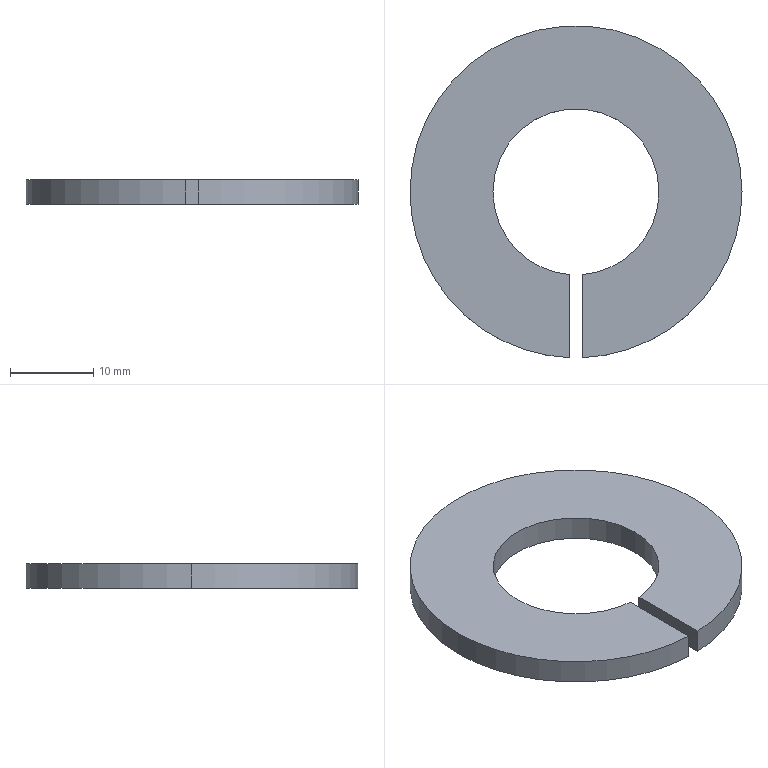Part | STEP file | qnSceond3_2 | 1 solid | 10 faces | box 40 x 39.986 x 3 mm | volume 2782 mm3 | cylinder 6 | plane 4 | commonest cylinder face diameters 20 x3 40 x3
STEP:
#1=CARTESIAN_POINT('',(0.,0.,0.));
#2=DIRECTION('',(0.,0.,1.));
#3=DIRECTION('',(1.,0.,0.));
#4=AXIS2_PLACEMENT_3D('',#1,#2,#3);
#5=CARTESIAN_POINT('',(20.,0.,8.));
#6=VERTEX_POINT('',#5);
#7=CARTESIAN_POINT('',(-20.,0.,8.));
#8=VERTEX_POINT('',#7);
#9=CARTESIAN_POINT('',(0.,0.,8.));
#10=DIRECTION('',(0.,0.,1.));
#11=DIRECTION('',(-1.,0.,0.));
#12=AXIS2_PLACEMENT_3D('',#9,#10,#11);
#13=CIRCLE('',#12,20.);
#14=CARTESIAN_POINT('',(0.,0.,6.5));
#15=DIRECTION('',(0.,0.,-1.));
#16=DIRECTION('',(-1.,0.,0.));
#17=AXIS2_PLACEMENT_3D('',#14,#15,#16);
#18=CYLINDRICAL_SURFACE('',#17,20.);
#19=CARTESIAN_POINT('',(6.283,-1.5));
#20=DIRECTION('',(-1.,0.));
#21=VECTOR('',#20,1.);
#22=LINE('',#19,#21);
#23=(GEOMETRIC_REPRESENTATION_CONTEXT(2)PARAMETRIC_REPRESENTATION_CONTEXT()REPRESENTATION_CONTEXT('',''));
#24=DEFINITIONAL_REPRESENTATION('',(#22),#23);
#25=PCURVE('',#18,#24);
#26=CARTESIAN_POINT('',(0.,15.,8.));
#27=DIRECTION('',(0.,0.,1.));
#28=DIRECTION('',(1.,0.,0.));
#29=AXIS2_PLACEMENT_3D('',#26,#27,#28);
#30=PLANE('',#29);
#31=CARTESIAN_POINT('',(0.,-15.));
#32=DIRECTION('',(-1.,0.));
#33=AXIS2_PLACEMENT_2D('',#31,#32);
#34=CIRCLE('',#33,20.);
#35=(GEOMETRIC_REPRESENTATION_CONTEXT(2)PARAMETRIC_REPRESENTATION_CONTEXT()REPRESENTATION_CONTEXT('',''));
#36=DEFINITIONAL_REPRESENTATION('',(#34),#35);
#37=PCURVE('',#30,#36);
#38=SURFACE_CURVE('',#13,(#25,#37),.PCURVE_S1.);
#39=EDGE_CURVE('',#6,#8,#38,.T.);
#40=ORIENTED_EDGE('',*,*,#39,.F.);
#41=CARTESIAN_POINT('',(20.,0.,5.));
#42=VERTEX_POINT('',#41);
#43=CARTESIAN_POINT('',(20.,0.,6.5));
#44=DIRECTION('',(0.,0.,-1.));
#45=VECTOR('',#44,1.);
#46=LINE('',#43,#45);
#47=CARTESIAN_POINT('',(3.142,0.));
#48=DIRECTION('',(0.,1.));
#49=VECTOR('',#48,1.);
#50=LINE('',#47,#49);
#51=(GEOMETRIC_REPRESENTATION_CONTEXT(2)PARAMETRIC_REPRESENTATION_CONTEXT()REPRESENTATION_CONTEXT('',''));
#52=DEFINITIONAL_REPRESENTATION('',(#50),#51);
#53=PCURVE('',#18,#52);
#54=CARTESIAN_POINT('',(0.,0.,6.5));
#55=DIRECTION('',(0.,0.,-1.));
#56=DIRECTION('',(-1.,0.,0.));
#57=AXIS2_PLACEMENT_3D('',#54,#55,#56);
#58=CYLINDRICAL_SURFACE('',#57,20.);
#59=CARTESIAN_POINT('',(3.142,0.));
#60=DIRECTION('',(0.,1.));
#61=VECTOR('',#60,1.);
#62=LINE('',#59,#61);
#63=(GEOMETRIC_REPRESENTATION_CONTEXT(2)PARAMETRIC_REPRESENTATION_CONTEXT()REPRESENTATION_CONTEXT('',''));
#64=DEFINITIONAL_REPRESENTATION('',(#62),#63);
#65=PCURVE('',#58,#64);
#66=SURFACE_CURVE('',#46,(#53,#65),.PCURVE_S1.);
#67=EDGE_CURVE('',#6,#42,#66,.T.);
#68=ORIENTED_EDGE('',*,*,#67,.T.);
#69=CARTESIAN_POINT('',(-20.,0.,5.));
#70=VERTEX_POINT('',#69);
#71=CARTESIAN_POINT('',(0.,0.,5.));
#72=DIRECTION('',(0.,0.,1.));
#73=DIRECTION('',(-1.,0.,0.));
#74=AXIS2_PLACEMENT_3D('',#71,#72,#73);
#75=CIRCLE('',#74,20.);
#76=CARTESIAN_POINT('',(6.283,1.5));
#77=DIRECTION('',(-1.,0.));
#78=VECTOR('',#77,1.);
#79=LINE('',#76,#78);
#80=(GEOMETRIC_REPRESENTATION_CONTEXT(2)PARAMETRIC_REPRESENTATION_CONTEXT()REPRESENTATION_CONTEXT('',''));
#81=DEFINITIONAL_REPRESENTATION('',(#79),#80);
#82=PCURVE('',#18,#81);
#83=CARTESIAN_POINT('',(0.,15.,5.));
#84=DIRECTION('',(0.,0.,-1.));
#85=DIRECTION('',(-1.,0.,0.));
#86=AXIS2_PLACEMENT_3D('',#83,#84,#85);
#87=PLANE('',#86);
#88=CARTESIAN_POINT('',(20.,-15.));
#89=CARTESIAN_POINT('',(20.,-49.641));
#90=CARTESIAN_POINT('',(-10.,-32.321));
#91=CARTESIAN_POINT('',(-40.,-15.));
#92=CARTESIAN_POINT('',(-10.,2.321));
#93=CARTESIAN_POINT('',(20.,19.641));
#94=CARTESIAN_POINT('',(20.,-15.));
#95=(BOUNDED_CURVE()B_SPLINE_CURVE(2,(#88,#89,#90,#91,#92,#93,#94),.UNSPECIFIED.,.T.,.F.)B_SPLINE_CURVE_WITH_KNOTS((1,2,2,2,2,1),(-2.094,0.,2.094,4.189,6.283,8.378),.UNSPECIFIED.)CURVE()GEOMETRIC_REPRESENTATION_ITEM()RATIONAL_B_SPLINE_CURVE((1.,0.5,1.,0.5,1.,0.5,1.))REPRESENTATION_ITEM(''));
#96=(GEOMETRIC_REPRESENTATION_CONTEXT(2)PARAMETRIC_REPRESENTATION_CONTEXT()REPRESENTATION_CONTEXT('',''));
#97=DEFINITIONAL_REPRESENTATION('',(#95),#96);
#98=PCURVE('',#87,#97);
#99=SURFACE_CURVE('',#75,(#82,#98),.PCURVE_S1.);
#100=EDGE_CURVE('',#42,#70,#99,.T.);
#101=ORIENTED_EDGE('',*,*,#100,.T.);
#102=CARTESIAN_POINT('',(-20.,0.,6.5));
#103=DIRECTION('',(0.,0.,-1.));
#104=VECTOR('',#103,1.);
#105=LINE('',#102,#104);
#106=CARTESIAN_POINT('',(0.,0.));
#107=DIRECTION('',(0.,1.));
#108=VECTOR('',#107,1.);
#109=LINE('',#106,#108);
#110=(GEOMETRIC_REPRESENTATION_CONTEXT(2)PARAMETRIC_REPRESENTATION_CONTEXT()REPRESENTATION_CONTEXT('',''));
#111=DEFINITIONAL_REPRESENTATION('',(#109),#110);
#112=PCURVE('',#18,#111);
#113=CARTESIAN_POINT('',(0.,0.,6.5));
#114=DIRECTION('',(0.,0.,-1.));
#115=DIRECTION('',(-1.,0.,0.));
#116=AXIS2_PLACEMENT_3D('',#113,#114,#115);
#117=CYLINDRICAL_SURFACE('',#116,20.);
#118=CARTESIAN_POINT('',(6.283,0.));
#119=DIRECTION('',(0.,1.));
#120=VECTOR('',#119,1.);
#121=LINE('',#118,#120);
#122=(GEOMETRIC_REPRESENTATION_CONTEXT(2)PARAMETRIC_REPRESENTATION_CONTEXT()REPRESENTATION_CONTEXT('',''));
#123=DEFINITIONAL_REPRESENTATION('',(#121),#122);
#124=PCURVE('',#117,#123);
#125=SURFACE_CURVE('',#105,(#112,#124),.PCURVE_S1.);
#126=EDGE_CURVE('',#8,#70,#125,.T.);
#127=ORIENTED_EDGE('',*,*,#126,.F.);
#128=EDGE_LOOP('',(#40,#68,#101,#127));
#129=FACE_BOUND('',#128,.T.);
#130=ADVANCED_FACE('',(#129),#18,.T.);
#131=CARTESIAN_POINT('',(-0.75,-19.986,8.));
#132=VERTEX_POINT('',#131);
#133=CARTESIAN_POINT('',(0.,0.,8.));
#134=DIRECTION('',(0.,0.,1.));
#135=DIRECTION('',(-1.,0.,0.));
#136=AXIS2_PLACEMENT_3D('',#133,#134,#135);
#137=CIRCLE('',#136,20.);
#138=CARTESIAN_POINT('',(6.283,-1.5));
#139=DIRECTION('',(-1.,0.));
#140=VECTOR('',#139,1.);
#141=LINE('',#138,#140);
#142=(GEOMETRIC_REPRESENTATION_CONTEXT(2)PARAMETRIC_REPRESENTATION_CONTEXT()REPRESENTATION_CONTEXT('',''));
#143=DEFINITIONAL_REPRESENTATION('',(#141),#142);
#144=PCURVE('',#117,#143);
#145=CARTESIAN_POINT('',(0.,-15.));
#146=DIRECTION('',(-1.,0.));
#147=AXIS2_PLACEMENT_2D('',#145,#146);
#148=CIRCLE('',#147,20.);
#149=(GEOMETRIC_REPRESENTATION_CONTEXT(2)PARAMETRIC_REPRESENTATION_CONTEXT()REPRESENTATION_CONTEXT('',''));
#150=DEFINITIONAL_REPRESENTATION('',(#148),#149);
#151=PCURVE('',#30,#150);
#152=SURFACE_CURVE('',#137,(#144,#151),.PCURVE_S1.);
#153=EDGE_CURVE('',#8,#132,#152,.T.);
#154=ORIENTED_EDGE('',*,*,#153,.F.);
#155=ORIENTED_EDGE('',*,*,#126,.T.);
#156=CARTESIAN_POINT('',(-0.75,-19.986,5.));
#157=VERTEX_POINT('',#156);
#158=CARTESIAN_POINT('',(0.,0.,5.));
#159=DIRECTION('',(0.,0.,1.));
#160=DIRECTION('',(-1.,0.,0.));
#161=AXIS2_PLACEMENT_3D('',#158,#159,#160);
#162=CIRCLE('',#161,20.);
#163=CARTESIAN_POINT('',(6.283,1.5));
#164=DIRECTION('',(-1.,0.));
#165=VECTOR('',#164,1.);
#166=LINE('',#163,#165);
#167=(GEOMETRIC_REPRESENTATION_CONTEXT(2)PARAMETRIC_REPRESENTATION_CONTEXT()REPRESENTATION_CONTEXT('',''));
#168=DEFINITIONAL_REPRESENTATION('',(#166),#167);
#169=PCURVE('',#117,#168);
#170=CARTESIAN_POINT('',(20.,-15.));
#171=CARTESIAN_POINT('',(20.,-49.641));
#172=CARTESIAN_POINT('',(-10.,-32.321));
#173=CARTESIAN_POINT('',(-40.,-15.));
#174=CARTESIAN_POINT('',(-10.,2.321));
#175=CARTESIAN_POINT('',(20.,19.641));
#176=CARTESIAN_POINT('',(20.,-15.));
#177=(BOUNDED_CURVE()B_SPLINE_CURVE(2,(#170,#171,#172,#173,#174,#175,#176),.UNSPECIFIED.,.T.,.F.)B_SPLINE_CURVE_WITH_KNOTS((1,2,2,2,2,1),(-2.094,0.,2.094,4.189,6.283,8.378),.UNSPECIFIED.)CURVE()GEOMETRIC_REPRESENTATION_ITEM()RATIONAL_B_SPLINE_CURVE((1.,0.5,1.,0.5,1.,0.5,1.))REPRESENTATION_ITEM(''));
#178=(GEOMETRIC_REPRESENTATION_CONTEXT(2)PARAMETRIC_REPRESENTATION_CONTEXT()REPRESENTATION_CONTEXT('',''));
#179=DEFINITIONAL_REPRESENTATION('',(#177),#178);
#180=PCURVE('',#87,#179);
#181=SURFACE_CURVE('',#162,(#169,#180),.PCURVE_S1.);
#182=EDGE_CURVE('',#70,#157,#181,.T.);
#183=ORIENTED_EDGE('',*,*,#182,.T.);
#184=CARTESIAN_POINT('',(-0.75,-19.986,6.5));
#185=DIRECTION('',(0.,0.,1.));
#186=VECTOR('',#185,1.);
#187=LINE('',#184,#186);
#188=CARTESIAN_POINT('',(4.75,0.));
#189=DIRECTION('',(0.,-1.));
#190=VECTOR('',#189,1.);
#191=LINE('',#188,#190);
#192=(GEOMETRIC_REPRESENTATION_CONTEXT(2)PARAMETRIC_REPRESENTATION_CONTEXT()REPRESENTATION_CONTEXT('',''));
#193=DEFINITIONAL_REPRESENTATION('',(#191),#192);
#194=PCURVE('',#117,#193);
#195=CARTESIAN_POINT('',(-0.75,-40.,5.));
#196=DIRECTION('',(-1.,0.,0.));
#197=DIRECTION('',(0.,0.,1.));
#198=AXIS2_PLACEMENT_3D('',#195,#196,#197);
#199=PLANE('',#198);
#200=CARTESIAN_POINT('',(1.5,20.014));
#201=DIRECTION('',(1.,0.));
#202=VECTOR('',#201,1.);
#203=LINE('',#200,#202);
#204=(GEOMETRIC_REPRESENTATION_CONTEXT(2)PARAMETRIC_REPRESENTATION_CONTEXT()REPRESENTATION_CONTEXT('',''));
#205=DEFINITIONAL_REPRESENTATION('',(#203),#204);
#206=PCURVE('',#199,#205);
#207=SURFACE_CURVE('',#187,(#194,#206),.PCURVE_S1.);
#208=EDGE_CURVE('',#157,#132,#207,.T.);
#209=ORIENTED_EDGE('',*,*,#208,.T.);
#210=EDGE_LOOP('',(#154,#155,#183,#209));
#211=FACE_BOUND('',#210,.T.);
#212=ADVANCED_FACE('',(#211),#117,.T.);
#213=CARTESIAN_POINT('',(0.75,-9.972,5.));
#214=VERTEX_POINT('',#213);
#215=CARTESIAN_POINT('',(0.75,-9.972,8.));
#216=VERTEX_POINT('',#215);
#217=CARTESIAN_POINT('',(0.75,-9.972,5.));
#218=DIRECTION('',(0.,0.,1.));
#219=VECTOR('',#218,1.);
#220=LINE('',#217,#219);
#221=CARTESIAN_POINT('',(0.,0.,6.5));
#222=DIRECTION('',(0.,0.,-1.));
#223=DIRECTION('',(-1.,0.,0.));
#224=AXIS2_PLACEMENT_3D('',#221,#222,#223);
#225=CYLINDRICAL_SURFACE('',#224,10.);
#226=CARTESIAN_POINT('',(4.637,1.5));
#227=DIRECTION('',(0.,-1.));
#228=VECTOR('',#227,1.);
#229=LINE('',#226,#228);
#230=(GEOMETRIC_REPRESENTATION_CONTEXT(2)PARAMETRIC_REPRESENTATION_CONTEXT()REPRESENTATION_CONTEXT('',''));
#231=DEFINITIONAL_REPRESENTATION('',(#229),#230);
#232=PCURVE('',#225,#231);
#233=CARTESIAN_POINT('',(0.75,0.,5.));
#234=DIRECTION('',(1.,0.,0.));
#235=DIRECTION('',(0.,0.,-1.));
#236=AXIS2_PLACEMENT_3D('',#233,#234,#235);
#237=PLANE('',#236);
#238=CARTESIAN_POINT('',(0.,-9.972));
#239=DIRECTION('',(-1.,0.));
#240=VECTOR('',#239,1.);
#241=LINE('',#238,#240);
#242=(GEOMETRIC_REPRESENTATION_CONTEXT(2)PARAMETRIC_REPRESENTATION_CONTEXT()REPRESENTATION_CONTEXT('',''));
#243=DEFINITIONAL_REPRESENTATION('',(#241),#242);
#244=PCURVE('',#237,#243);
#245=SURFACE_CURVE('',#220,(#232,#244),.PCURVE_S1.);
#246=EDGE_CURVE('',#214,#216,#245,.T.);
#247=ORIENTED_EDGE('',*,*,#246,.F.);
#248=CARTESIAN_POINT('',(10.,0.,5.));
#249=VERTEX_POINT('',#248);
#250=CARTESIAN_POINT('',(0.,0.,5.));
#251=DIRECTION('',(0.,0.,1.));
#252=DIRECTION('',(-1.,0.,0.));
#253=AXIS2_PLACEMENT_3D('',#250,#251,#252);
#254=CIRCLE('',#253,10.);
#255=CARTESIAN_POINT('',(6.283,1.5));
#256=DIRECTION('',(-1.,0.));
#257=VECTOR('',#256,1.);
#258=LINE('',#255,#257);
#259=(GEOMETRIC_REPRESENTATION_CONTEXT(2)PARAMETRIC_REPRESENTATION_CONTEXT()REPRESENTATION_CONTEXT('',''));
#260=DEFINITIONAL_REPRESENTATION('',(#258),#259);
#261=PCURVE('',#225,#260);
#262=CARTESIAN_POINT('',(10.,-15.));
#263=CARTESIAN_POINT('',(10.,-32.321));
#264=CARTESIAN_POINT('',(-5.,-23.66));
#265=CARTESIAN_POINT('',(-20.,-15.));
#266=CARTESIAN_POINT('',(-5.,-6.34));
#267=CARTESIAN_POINT('',(10.,2.321));
#268=CARTESIAN_POINT('',(10.,-15.));
#269=(BOUNDED_CURVE()B_SPLINE_CURVE(2,(#262,#263,#264,#265,#266,#267,#268),.UNSPECIFIED.,.T.,.F.)B_SPLINE_CURVE_WITH_KNOTS((1,2,2,2,2,1),(-2.094,0.,2.094,4.189,6.283,8.378),.UNSPECIFIED.)CURVE()GEOMETRIC_REPRESENTATION_ITEM()RATIONAL_B_SPLINE_CURVE((1.,0.5,1.,0.5,1.,0.5,1.))REPRESENTATION_ITEM(''));
#270=(GEOMETRIC_REPRESENTATION_CONTEXT(2)PARAMETRIC_REPRESENTATION_CONTEXT()REPRESENTATION_CONTEXT('',''));
#271=DEFINITIONAL_REPRESENTATION('',(#269),#270);
#272=PCURVE('',#87,#271);
#273=SURFACE_CURVE('',#254,(#261,#272),.PCURVE_S1.);
#274=EDGE_CURVE('',#214,#249,#273,.T.);
#275=ORIENTED_EDGE('',*,*,#274,.T.);
#276=CARTESIAN_POINT('',(10.,0.,8.));
#277=VERTEX_POINT('',#276);
#278=CARTESIAN_POINT('',(10.,0.,6.5));
#279=DIRECTION('',(0.,0.,-1.));
#280=VECTOR('',#279,1.);
#281=LINE('',#278,#280);
#282=CARTESIAN_POINT('',(3.142,0.));
#283=DIRECTION('',(0.,1.));
#284=VECTOR('',#283,1.);
#285=LINE('',#282,#284);
#286=(GEOMETRIC_REPRESENTATION_CONTEXT(2)PARAMETRIC_REPRESENTATION_CONTEXT()REPRESENTATION_CONTEXT('',''));
#287=DEFINITIONAL_REPRESENTATION('',(#285),#286);
#288=PCURVE('',#225,#287);
#289=CARTESIAN_POINT('',(0.,0.,6.5));
#290=DIRECTION('',(0.,0.,-1.));
#291=DIRECTION('',(-1.,0.,0.));
#292=AXIS2_PLACEMENT_3D('',#289,#290,#291);
#293=CYLINDRICAL_SURFACE('',#292,10.);
#294=CARTESIAN_POINT('',(3.142,0.));
#295=DIRECTION('',(0.,1.));
#296=VECTOR('',#295,1.);
#297=LINE('',#294,#296);
#298=(GEOMETRIC_REPRESENTATION_CONTEXT(2)PARAMETRIC_REPRESENTATION_CONTEXT()REPRESENTATION_CONTEXT('',''));
#299=DEFINITIONAL_REPRESENTATION('',(#297),#298);
#300=PCURVE('',#293,#299);
#301=SURFACE_CURVE('',#281,(#288,#300),.PCURVE_S1.);
#302=EDGE_CURVE('',#277,#249,#301,.T.);
#303=ORIENTED_EDGE('',*,*,#302,.F.);
#304=CARTESIAN_POINT('',(0.,0.,8.));
#305=DIRECTION('',(0.,0.,-1.));
#306=DIRECTION('',(-1.,0.,0.));
#307=AXIS2_PLACEMENT_3D('',#304,#305,#306);
#308=CIRCLE('',#307,10.);
#309=CARTESIAN_POINT('',(0.,-1.5));
#310=DIRECTION('',(1.,0.));
#311=VECTOR('',#310,1.);
#312=LINE('',#309,#311);
#313=(GEOMETRIC_REPRESENTATION_CONTEXT(2)PARAMETRIC_REPRESENTATION_CONTEXT()REPRESENTATION_CONTEXT('',''));
#314=DEFINITIONAL_REPRESENTATION('',(#312),#313);
#315=PCURVE('',#225,#314);
#316=CARTESIAN_POINT('',(-10.,-15.));
#317=CARTESIAN_POINT('',(-10.,2.321));
#318=CARTESIAN_POINT('',(5.,-6.34));
#319=CARTESIAN_POINT('',(20.,-15.));
#320=CARTESIAN_POINT('',(5.,-23.66));
#321=CARTESIAN_POINT('',(-10.,-32.321));
#322=CARTESIAN_POINT('',(-10.,-15.));
#323=(BOUNDED_CURVE()B_SPLINE_CURVE(2,(#316,#317,#318,#319,#320,#321,#322),.UNSPECIFIED.,.T.,.F.)B_SPLINE_CURVE_WITH_KNOTS((1,2,2,2,2,1),(-2.094,0.,2.094,4.189,6.283,8.378),.UNSPECIFIED.)CURVE()GEOMETRIC_REPRESENTATION_ITEM()RATIONAL_B_SPLINE_CURVE((1.,0.5,1.,0.5,1.,0.5,1.))REPRESENTATION_ITEM(''));
#324=(GEOMETRIC_REPRESENTATION_CONTEXT(2)PARAMETRIC_REPRESENTATION_CONTEXT()REPRESENTATION_CONTEXT('',''));
#325=DEFINITIONAL_REPRESENTATION('',(#323),#324);
#326=PCURVE('',#30,#325);
#327=SURFACE_CURVE('',#308,(#315,#326),.PCURVE_S1.);
#328=EDGE_CURVE('',#277,#216,#327,.T.);
#329=ORIENTED_EDGE('',*,*,#328,.T.);
#330=EDGE_LOOP('',(#247,#275,#303,#329));
#331=FACE_BOUND('',#330,.F.);
#332=ADVANCED_FACE('',(#331),#225,.F.);
#333=CARTESIAN_POINT('',(-10.,0.,5.));
#334=VERTEX_POINT('',#333);
#335=CARTESIAN_POINT('',(0.,0.,5.));
#336=DIRECTION('',(0.,0.,1.));
#337=DIRECTION('',(-1.,0.,0.));
#338=AXIS2_PLACEMENT_3D('',#335,#336,#337);
#339=CIRCLE('',#338,10.);
#340=CARTESIAN_POINT('',(6.283,1.5));
#341=DIRECTION('',(-1.,0.));
#342=VECTOR('',#341,1.);
#343=LINE('',#340,#342);
#344=(GEOMETRIC_REPRESENTATION_CONTEXT(2)PARAMETRIC_REPRESENTATION_CONTEXT()REPRESENTATION_CONTEXT('',''));
#345=DEFINITIONAL_REPRESENTATION('',(#343),#344);
#346=PCURVE('',#293,#345);
#347=CARTESIAN_POINT('',(10.,-15.));
#348=CARTESIAN_POINT('',(10.,-32.321));
#349=CARTESIAN_POINT('',(-5.,-23.66));
#350=CARTESIAN_POINT('',(-20.,-15.));
#351=CARTESIAN_POINT('',(-5.,-6.34));
#352=CARTESIAN_POINT('',(10.,2.321));
#353=CARTESIAN_POINT('',(10.,-15.));
#354=(BOUNDED_CURVE()B_SPLINE_CURVE(2,(#347,#348,#349,#350,#351,#352,#353),.UNSPECIFIED.,.T.,.F.)B_SPLINE_CURVE_WITH_KNOTS((1,2,2,2,2,1),(-2.094,0.,2.094,4.189,6.283,8.378),.UNSPECIFIED.)CURVE()GEOMETRIC_REPRESENTATION_ITEM()RATIONAL_B_SPLINE_CURVE((1.,0.5,1.,0.5,1.,0.5,1.))REPRESENTATION_ITEM(''));
#355=(GEOMETRIC_REPRESENTATION_CONTEXT(2)PARAMETRIC_REPRESENTATION_CONTEXT()REPRESENTATION_CONTEXT('',''));
#356=DEFINITIONAL_REPRESENTATION('',(#354),#355);
#357=PCURVE('',#87,#356);
#358=SURFACE_CURVE('',#339,(#346,#357),.PCURVE_S1.);
#359=EDGE_CURVE('',#249,#334,#358,.T.);
#360=ORIENTED_EDGE('',*,*,#359,.T.);
#361=CARTESIAN_POINT('',(-10.,0.,8.));
#362=VERTEX_POINT('',#361);
#363=CARTESIAN_POINT('',(-10.,0.,6.5));
#364=DIRECTION('',(0.,0.,-1.));
#365=VECTOR('',#364,1.);
#366=LINE('',#363,#365);
#367=CARTESIAN_POINT('',(0.,0.));
#368=DIRECTION('',(0.,1.));
#369=VECTOR('',#368,1.);
#370=LINE('',#367,#369);
#371=(GEOMETRIC_REPRESENTATION_CONTEXT(2)PARAMETRIC_REPRESENTATION_CONTEXT()REPRESENTATION_CONTEXT('',''));
#372=DEFINITIONAL_REPRESENTATION('',(#370),#371);
#373=PCURVE('',#293,#372);
#374=CARTESIAN_POINT('',(0.,0.,6.5));
#375=DIRECTION('',(0.,0.,-1.));
#376=DIRECTION('',(-1.,0.,0.));
#377=AXIS2_PLACEMENT_3D('',#374,#375,#376);
#378=CYLINDRICAL_SURFACE('',#377,10.);
#379=CARTESIAN_POINT('',(6.283,0.));
#380=DIRECTION('',(0.,1.));
#381=VECTOR('',#380,1.);
#382=LINE('',#379,#381);
#383=(GEOMETRIC_REPRESENTATION_CONTEXT(2)PARAMETRIC_REPRESENTATION_CONTEXT()REPRESENTATION_CONTEXT('',''));
#384=DEFINITIONAL_REPRESENTATION('',(#382),#383);
#385=PCURVE('',#378,#384);
#386=SURFACE_CURVE('',#366,(#373,#385),.PCURVE_S1.);
#387=EDGE_CURVE('',#362,#334,#386,.T.);
#388=ORIENTED_EDGE('',*,*,#387,.F.);
#389=CARTESIAN_POINT('',(0.,0.,8.));
#390=DIRECTION('',(0.,0.,-1.));
#391=DIRECTION('',(-1.,0.,0.));
#392=AXIS2_PLACEMENT_3D('',#389,#390,#391);
#393=CIRCLE('',#392,10.);
#394=CARTESIAN_POINT('',(0.,-1.5));
#395=DIRECTION('',(1.,0.));
#396=VECTOR('',#395,1.);
#397=LINE('',#394,#396);
#398=(GEOMETRIC_REPRESENTATION_CONTEXT(2)PARAMETRIC_REPRESENTATION_CONTEXT()REPRESENTATION_CONTEXT('',''));
#399=DEFINITIONAL_REPRESENTATION('',(#397),#398);
#400=PCURVE('',#293,#399);
#401=CARTESIAN_POINT('',(-10.,-15.));
#402=CARTESIAN_POINT('',(-10.,2.321));
#403=CARTESIAN_POINT('',(5.,-6.34));
#404=CARTESIAN_POINT('',(20.,-15.));
#405=CARTESIAN_POINT('',(5.,-23.66));
#406=CARTESIAN_POINT('',(-10.,-32.321));
#407=CARTESIAN_POINT('',(-10.,-15.));
#408=(BOUNDED_CURVE()B_SPLINE_CURVE(2,(#401,#402,#403,#404,#405,#406,#407),.UNSPECIFIED.,.T.,.F.)B_SPLINE_CURVE_WITH_KNOTS((1,2,2,2,2,1),(-2.094,0.,2.094,4.189,6.283,8.378),.UNSPECIFIED.)CURVE()GEOMETRIC_REPRESENTATION_ITEM()RATIONAL_B_SPLINE_CURVE((1.,0.5,1.,0.5,1.,0.5,1.))REPRESENTATION_ITEM(''));
#409=(GEOMETRIC_REPRESENTATION_CONTEXT(2)PARAMETRIC_REPRESENTATION_CONTEXT()REPRESENTATION_CONTEXT('',''));
#410=DEFINITIONAL_REPRESENTATION('',(#408),#409);
#411=PCURVE('',#30,#410);
#412=SURFACE_CURVE('',#393,(#400,#411),.PCURVE_S1.);
#413=EDGE_CURVE('',#362,#277,#412,.T.);
#414=ORIENTED_EDGE('',*,*,#413,.T.);
#415=ORIENTED_EDGE('',*,*,#302,.T.);
#416=EDGE_LOOP('',(#360,#388,#414,#415));
#417=FACE_BOUND('',#416,.F.);
#418=ADVANCED_FACE('',(#417),#293,.F.);
#419=CARTESIAN_POINT('',(0.75,-19.986,8.));
#420=VERTEX_POINT('',#419);
#421=CARTESIAN_POINT('',(0.,0.,8.));
#422=DIRECTION('',(0.,0.,1.));
#423=DIRECTION('',(-1.,0.,0.));
#424=AXIS2_PLACEMENT_3D('',#421,#422,#423);
#425=CIRCLE('',#424,20.);
#426=CARTESIAN_POINT('',(0.,-15.));
#427=DIRECTION('',(-1.,0.));
#428=AXIS2_PLACEMENT_2D('',#426,#427);
#429=CIRCLE('',#428,20.);
#430=(GEOMETRIC_REPRESENTATION_CONTEXT(2)PARAMETRIC_REPRESENTATION_CONTEXT()REPRESENTATION_CONTEXT('',''));
#431=DEFINITIONAL_REPRESENTATION('',(#429),#430);
#432=PCURVE('',#30,#431);
#433=CARTESIAN_POINT('',(6.283,-1.5));
#434=DIRECTION('',(-1.,0.));
#435=VECTOR('',#434,1.);
#436=LINE('',#433,#435);
#437=(GEOMETRIC_REPRESENTATION_CONTEXT(2)PARAMETRIC_REPRESENTATION_CONTEXT()REPRESENTATION_CONTEXT('',''));
#438=DEFINITIONAL_REPRESENTATION('',(#436),#437);
#439=PCURVE('',#58,#438);
#440=SURFACE_CURVE('',#425,(#432,#439),.PCURVE_S1.);
#441=EDGE_CURVE('',#420,#6,#440,.T.);
#442=ORIENTED_EDGE('',*,*,#441,.T.);
#443=ORIENTED_EDGE('',*,*,#39,.T.);
#444=ORIENTED_EDGE('',*,*,#153,.T.);
#445=CARTESIAN_POINT('',(-0.75,-9.972,8.));
#446=VERTEX_POINT('',#445);
#447=CARTESIAN_POINT('',(-0.75,15.,8.));
#448=DIRECTION('',(0.,1.,0.));
#449=VECTOR('',#448,1.);
#450=LINE('',#447,#449);
#451=CARTESIAN_POINT('',(-0.75,0.));
#452=DIRECTION('',(0.,1.));
#453=VECTOR('',#452,1.);
#454=LINE('',#451,#453);
#455=(GEOMETRIC_REPRESENTATION_CONTEXT(2)PARAMETRIC_REPRESENTATION_CONTEXT()REPRESENTATION_CONTEXT('',''));
#456=DEFINITIONAL_REPRESENTATION('',(#454),#455);
#457=PCURVE('',#30,#456);
#458=CARTESIAN_POINT('',(3.,55.));
#459=DIRECTION('',(0.,1.));
#460=VECTOR('',#459,1.);
#461=LINE('',#458,#460);
#462=(GEOMETRIC_REPRESENTATION_CONTEXT(2)PARAMETRIC_REPRESENTATION_CONTEXT()REPRESENTATION_CONTEXT('',''));
#463=DEFINITIONAL_REPRESENTATION('',(#461),#462);
#464=PCURVE('',#199,#463);
#465=SURFACE_CURVE('',#450,(#457,#464),.PCURVE_S1.);
#466=EDGE_CURVE('',#132,#446,#465,.T.);
#467=ORIENTED_EDGE('',*,*,#466,.T.);
#468=CARTESIAN_POINT('',(0.,0.,8.));
#469=DIRECTION('',(0.,0.,-1.));
#470=DIRECTION('',(-1.,0.,0.));
#471=AXIS2_PLACEMENT_3D('',#468,#469,#470);
#472=CIRCLE('',#471,10.);
#473=CARTESIAN_POINT('',(-10.,-15.));
#474=CARTESIAN_POINT('',(-10.,2.321));
#475=CARTESIAN_POINT('',(5.,-6.34));
#476=CARTESIAN_POINT('',(20.,-15.));
#477=CARTESIAN_POINT('',(5.,-23.66));
#478=CARTESIAN_POINT('',(-10.,-32.321));
#479=CARTESIAN_POINT('',(-10.,-15.));
#480=(BOUNDED_CURVE()B_SPLINE_CURVE(2,(#473,#474,#475,#476,#477,#478,#479),.UNSPECIFIED.,.T.,.F.)B_SPLINE_CURVE_WITH_KNOTS((1,2,2,2,2,1),(-2.094,0.,2.094,4.189,6.283,8.378),.UNSPECIFIED.)CURVE()GEOMETRIC_REPRESENTATION_ITEM()RATIONAL_B_SPLINE_CURVE((1.,0.5,1.,0.5,1.,0.5,1.))REPRESENTATION_ITEM(''));
#481=(GEOMETRIC_REPRESENTATION_CONTEXT(2)PARAMETRIC_REPRESENTATION_CONTEXT()REPRESENTATION_CONTEXT('',''));
#482=DEFINITIONAL_REPRESENTATION('',(#480),#481);
#483=PCURVE('',#30,#482);
#484=CARTESIAN_POINT('',(0.,-1.5));
#485=DIRECTION('',(1.,0.));
#486=VECTOR('',#485,1.);
#487=LINE('',#484,#486);
#488=(GEOMETRIC_REPRESENTATION_CONTEXT(2)PARAMETRIC_REPRESENTATION_CONTEXT()REPRESENTATION_CONTEXT('',''));
#489=DEFINITIONAL_REPRESENTATION('',(#487),#488);
#490=PCURVE('',#378,#489);
#491=SURFACE_CURVE('',#472,(#483,#490),.PCURVE_S1.);
#492=EDGE_CURVE('',#446,#362,#491,.T.);
#493=ORIENTED_EDGE('',*,*,#492,.T.);
#494=ORIENTED_EDGE('',*,*,#413,.T.);
#495=ORIENTED_EDGE('',*,*,#328,.T.);
#496=CARTESIAN_POINT('',(0.75,15.,8.));
#497=DIRECTION('',(0.,-1.,0.));
#498=VECTOR('',#497,1.);
#499=LINE('',#496,#498);
#500=CARTESIAN_POINT('',(0.75,0.));
#501=DIRECTION('',(0.,-1.));
#502=VECTOR('',#501,1.);
#503=LINE('',#500,#502);
#504=(GEOMETRIC_REPRESENTATION_CONTEXT(2)PARAMETRIC_REPRESENTATION_CONTEXT()REPRESENTATION_CONTEXT('',''));
#505=DEFINITIONAL_REPRESENTATION('',(#503),#504);
#506=PCURVE('',#30,#505);
#507=CARTESIAN_POINT('',(-3.,15.));
#508=DIRECTION('',(0.,-1.));
#509=VECTOR('',#508,1.);
#510=LINE('',#507,#509);
#511=(GEOMETRIC_REPRESENTATION_CONTEXT(2)PARAMETRIC_REPRESENTATION_CONTEXT()REPRESENTATION_CONTEXT('',''));
#512=DEFINITIONAL_REPRESENTATION('',(#510),#511);
#513=PCURVE('',#237,#512);
#514=SURFACE_CURVE('',#499,(#506,#513),.PCURVE_S1.);
#515=EDGE_CURVE('',#216,#420,#514,.T.);
#516=ORIENTED_EDGE('',*,*,#515,.T.);
#517=EDGE_LOOP('',(#442,#443,#444,#467,#493,#494,#495,#516));
#518=FACE_BOUND('',#517,.T.);
#519=ADVANCED_FACE('',(#518),#30,.T.);
#520=ORIENTED_EDGE('',*,*,#67,.F.);
#521=ORIENTED_EDGE('',*,*,#441,.F.);
#522=CARTESIAN_POINT('',(0.75,-19.986,5.));
#523=VERTEX_POINT('',#522);
#524=CARTESIAN_POINT('',(0.75,-19.986,6.5));
#525=DIRECTION('',(0.,0.,-1.));
#526=VECTOR('',#525,1.);
#527=LINE('',#524,#526);
#528=CARTESIAN_POINT('',(4.675,0.));
#529=DIRECTION('',(0.,1.));
#530=VECTOR('',#529,1.);
#531=LINE('',#528,#530);
#532=(GEOMETRIC_REPRESENTATION_CONTEXT(2)PARAMETRIC_REPRESENTATION_CONTEXT()REPRESENTATION_CONTEXT('',''));
#533=DEFINITIONAL_REPRESENTATION('',(#531),#532);
#534=PCURVE('',#58,#533);
#535=CARTESIAN_POINT('',(-1.5,-19.986));
#536=DIRECTION('',(1.,0.));
#537=VECTOR('',#536,1.);
#538=LINE('',#535,#537);
#539=(GEOMETRIC_REPRESENTATION_CONTEXT(2)PARAMETRIC_REPRESENTATION_CONTEXT()REPRESENTATION_CONTEXT('',''));
#540=DEFINITIONAL_REPRESENTATION('',(#538),#539);
#541=PCURVE('',#237,#540);
#542=SURFACE_CURVE('',#527,(#534,#541),.PCURVE_S1.);
#543=EDGE_CURVE('',#420,#523,#542,.T.);
#544=ORIENTED_EDGE('',*,*,#543,.T.);
#545=CARTESIAN_POINT('',(0.,0.,5.));
#546=DIRECTION('',(0.,0.,1.));
#547=DIRECTION('',(-1.,0.,0.));
#548=AXIS2_PLACEMENT_3D('',#545,#546,#547);
#549=CIRCLE('',#548,20.);
#550=CARTESIAN_POINT('',(6.283,1.5));
#551=DIRECTION('',(-1.,0.));
#552=VECTOR('',#551,1.);
#553=LINE('',#550,#552);
#554=(GEOMETRIC_REPRESENTATION_CONTEXT(2)PARAMETRIC_REPRESENTATION_CONTEXT()REPRESENTATION_CONTEXT('',''));
#555=DEFINITIONAL_REPRESENTATION('',(#553),#554);
#556=PCURVE('',#58,#555);
#557=CARTESIAN_POINT('',(20.,-15.));
#558=CARTESIAN_POINT('',(20.,-49.641));
#559=CARTESIAN_POINT('',(-10.,-32.321));
#560=CARTESIAN_POINT('',(-40.,-15.));
#561=CARTESIAN_POINT('',(-10.,2.321));
#562=CARTESIAN_POINT('',(20.,19.641));
#563=CARTESIAN_POINT('',(20.,-15.));
#564=(BOUNDED_CURVE()B_SPLINE_CURVE(2,(#557,#558,#559,#560,#561,#562,#563),.UNSPECIFIED.,.T.,.F.)B_SPLINE_CURVE_WITH_KNOTS((1,2,2,2,2,1),(-2.094,0.,2.094,4.189,6.283,8.378),.UNSPECIFIED.)CURVE()GEOMETRIC_REPRESENTATION_ITEM()RATIONAL_B_SPLINE_CURVE((1.,0.5,1.,0.5,1.,0.5,1.))REPRESENTATION_ITEM(''));
#565=(GEOMETRIC_REPRESENTATION_CONTEXT(2)PARAMETRIC_REPRESENTATION_CONTEXT()REPRESENTATION_CONTEXT('',''));
#566=DEFINITIONAL_REPRESENTATION('',(#564),#565);
#567=PCURVE('',#87,#566);
#568=SURFACE_CURVE('',#549,(#556,#567),.PCURVE_S1.);
#569=EDGE_CURVE('',#523,#42,#568,.T.);
#570=ORIENTED_EDGE('',*,*,#569,.T.);
#571=EDGE_LOOP('',(#520,#521,#544,#570));
#572=FACE_BOUND('',#571,.T.);
#573=ADVANCED_FACE('',(#572),#58,.T.);
#574=CARTESIAN_POINT('',(0.75,0.,5.));
#575=DIRECTION('',(0.,1.,0.));
#576=VECTOR('',#575,1.);
#577=LINE('',#574,#576);
#578=CARTESIAN_POINT('',(0.,0.));
#579=DIRECTION('',(0.,1.));
#580=VECTOR('',#579,1.);
#581=LINE('',#578,#580);
#582=(GEOMETRIC_REPRESENTATION_CONTEXT(2)PARAMETRIC_REPRESENTATION_CONTEXT()REPRESENTATION_CONTEXT('',''));
#583=DEFINITIONAL_REPRESENTATION('',(#581),#582);
#584=PCURVE('',#237,#583);
#585=CARTESIAN_POINT('',(-0.75,-15.));
#586=DIRECTION('',(0.,1.));
#587=VECTOR('',#586,1.);
#588=LINE('',#585,#587);
#589=(GEOMETRIC_REPRESENTATION_CONTEXT(2)PARAMETRIC_REPRESENTATION_CONTEXT()REPRESENTATION_CONTEXT('',''));
#590=DEFINITIONAL_REPRESENTATION('',(#588),#589);
#591=PCURVE('',#87,#590);
#592=SURFACE_CURVE('',#577,(#584,#591),.PCURVE_S1.);
#593=EDGE_CURVE('',#523,#214,#592,.T.);
#594=ORIENTED_EDGE('',*,*,#593,.F.);
#595=ORIENTED_EDGE('',*,*,#543,.F.);
#596=ORIENTED_EDGE('',*,*,#515,.F.);
#597=ORIENTED_EDGE('',*,*,#246,.F.);
#598=EDGE_LOOP('',(#594,#595,#596,#597));
#599=FACE_BOUND('',#598,.T.);
#600=ADVANCED_FACE('',(#599),#237,.F.);
#601=CARTESIAN_POINT('',(-0.75,-9.972,5.));
#602=VERTEX_POINT('',#601);
#603=CARTESIAN_POINT('',(0.,0.,5.));
#604=DIRECTION('',(0.,0.,1.));
#605=DIRECTION('',(-1.,0.,0.));
#606=AXIS2_PLACEMENT_3D('',#603,#604,#605);
#607=CIRCLE('',#606,10.);
#608=CARTESIAN_POINT('',(6.283,1.5));
#609=DIRECTION('',(-1.,0.));
#610=VECTOR('',#609,1.);
#611=LINE('',#608,#610);
#612=(GEOMETRIC_REPRESENTATION_CONTEXT(2)PARAMETRIC_REPRESENTATION_CONTEXT()REPRESENTATION_CONTEXT('',''));
#613=DEFINITIONAL_REPRESENTATION('',(#611),#612);
#614=PCURVE('',#378,#613);
#615=CARTESIAN_POINT('',(10.,-15.));
#616=CARTESIAN_POINT('',(10.,-32.321));
#617=CARTESIAN_POINT('',(-5.,-23.66));
#618=CARTESIAN_POINT('',(-20.,-15.));
#619=CARTESIAN_POINT('',(-5.,-6.34));
#620=CARTESIAN_POINT('',(10.,2.321));
#621=CARTESIAN_POINT('',(10.,-15.));
#622=(BOUNDED_CURVE()B_SPLINE_CURVE(2,(#615,#616,#617,#618,#619,#620,#621),.UNSPECIFIED.,.T.,.F.)B_SPLINE_CURVE_WITH_KNOTS((1,2,2,2,2,1),(-2.094,0.,2.094,4.189,6.283,8.378),.UNSPECIFIED.)CURVE()GEOMETRIC_REPRESENTATION_ITEM()RATIONAL_B_SPLINE_CURVE((1.,0.5,1.,0.5,1.,0.5,1.))REPRESENTATION_ITEM(''));
#623=(GEOMETRIC_REPRESENTATION_CONTEXT(2)PARAMETRIC_REPRESENTATION_CONTEXT()REPRESENTATION_CONTEXT('',''));
#624=DEFINITIONAL_REPRESENTATION('',(#622),#623);
#625=PCURVE('',#87,#624);
#626=SURFACE_CURVE('',#607,(#614,#625),.PCURVE_S1.);
#627=EDGE_CURVE('',#334,#602,#626,.T.);
#628=ORIENTED_EDGE('',*,*,#627,.T.);
#629=CARTESIAN_POINT('',(-0.75,-9.972,6.5));
#630=DIRECTION('',(0.,0.,1.));
#631=VECTOR('',#630,1.);
#632=LINE('',#629,#631);
#633=CARTESIAN_POINT('',(4.787,0.));
#634=DIRECTION('',(0.,-1.));
#635=VECTOR('',#634,1.);
#636=LINE('',#633,#635);
#637=(GEOMETRIC_REPRESENTATION_CONTEXT(2)PARAMETRIC_REPRESENTATION_CONTEXT()REPRESENTATION_CONTEXT('',''));
#638=DEFINITIONAL_REPRESENTATION('',(#636),#637);
#639=PCURVE('',#378,#638);
#640=CARTESIAN_POINT('',(1.5,30.028));
#641=DIRECTION('',(1.,0.));
#642=VECTOR('',#641,1.);
#643=LINE('',#640,#642);
#644=(GEOMETRIC_REPRESENTATION_CONTEXT(2)PARAMETRIC_REPRESENTATION_CONTEXT()REPRESENTATION_CONTEXT('',''));
#645=DEFINITIONAL_REPRESENTATION('',(#643),#644);
#646=PCURVE('',#199,#645);
#647=SURFACE_CURVE('',#632,(#639,#646),.PCURVE_S1.);
#648=EDGE_CURVE('',#602,#446,#647,.T.);
#649=ORIENTED_EDGE('',*,*,#648,.T.);
#650=ORIENTED_EDGE('',*,*,#492,.T.);
#651=ORIENTED_EDGE('',*,*,#387,.T.);
#652=EDGE_LOOP('',(#628,#649,#650,#651));
#653=FACE_BOUND('',#652,.F.);
#654=ADVANCED_FACE('',(#653),#378,.F.);
#655=ORIENTED_EDGE('',*,*,#466,.F.);
#656=ORIENTED_EDGE('',*,*,#208,.F.);
#657=CARTESIAN_POINT('',(-0.75,-40.,5.));
#658=DIRECTION('',(0.,-1.,0.));
#659=VECTOR('',#658,1.);
#660=LINE('',#657,#659);
#661=CARTESIAN_POINT('',(0.,0.));
#662=DIRECTION('',(0.,-1.));
#663=VECTOR('',#662,1.);
#664=LINE('',#661,#663);
#665=(GEOMETRIC_REPRESENTATION_CONTEXT(2)PARAMETRIC_REPRESENTATION_CONTEXT()REPRESENTATION_CONTEXT('',''));
#666=DEFINITIONAL_REPRESENTATION('',(#664),#665);
#667=PCURVE('',#199,#666);
#668=CARTESIAN_POINT('',(0.75,-55.));
#669=DIRECTION('',(0.,-1.));
#670=VECTOR('',#669,1.);
#671=LINE('',#668,#670);
#672=(GEOMETRIC_REPRESENTATION_CONTEXT(2)PARAMETRIC_REPRESENTATION_CONTEXT()REPRESENTATION_CONTEXT('',''));
#673=DEFINITIONAL_REPRESENTATION('',(#671),#672);
#674=PCURVE('',#87,#673);
#675=SURFACE_CURVE('',#660,(#667,#674),.PCURVE_S1.);
#676=EDGE_CURVE('',#602,#157,#675,.T.);
#677=ORIENTED_EDGE('',*,*,#676,.F.);
#678=ORIENTED_EDGE('',*,*,#648,.T.);
#679=EDGE_LOOP('',(#655,#656,#677,#678));
#680=FACE_BOUND('',#679,.T.);
#681=ADVANCED_FACE('',(#680),#199,.F.);
#682=ORIENTED_EDGE('',*,*,#274,.T.);
#683=ORIENTED_EDGE('',*,*,#359,.T.);
#684=ORIENTED_EDGE('',*,*,#627,.T.);
#685=ORIENTED_EDGE('',*,*,#676,.T.);
#686=ORIENTED_EDGE('',*,*,#182,.F.);
#687=ORIENTED_EDGE('',*,*,#100,.F.);
#688=ORIENTED_EDGE('',*,*,#569,.F.);
#689=ORIENTED_EDGE('',*,*,#593,.T.);
#690=EDGE_LOOP('',(#682,#683,#684,#685,#686,#687,#688,#689));
#691=FACE_BOUND('',#690,.T.);
#692=ADVANCED_FACE('',(#691),#87,.T.);
#693=CLOSED_SHELL('',(#130,#212,#332,#418,#519,#573,#600,#654,#681,#692));
#694=MANIFOLD_SOLID_BREP('',#693);
#695=(LENGTH_UNIT()NAMED_UNIT(*)SI_UNIT(.MILLI.,.METRE.));
#696=UNCERTAINTY_MEASURE_WITH_UNIT(LENGTH_MEASURE(0.0000001),#695,'','');
#697=(NAMED_UNIT(*)PLANE_ANGLE_UNIT()SI_UNIT($,.RADIAN.));
#698=(NAMED_UNIT(*)SI_UNIT($,.STERADIAN.)SOLID_ANGLE_UNIT());
#699=(GEOMETRIC_REPRESENTATION_CONTEXT(3)GLOBAL_UNCERTAINTY_ASSIGNED_CONTEXT((#696))GLOBAL_UNIT_ASSIGNED_CONTEXT((#695,#697,#698))REPRESENTATION_CONTEXT('',''));
#700=ADVANCED_BREP_SHAPE_REPRESENTATION('',(#4,#694),#699);